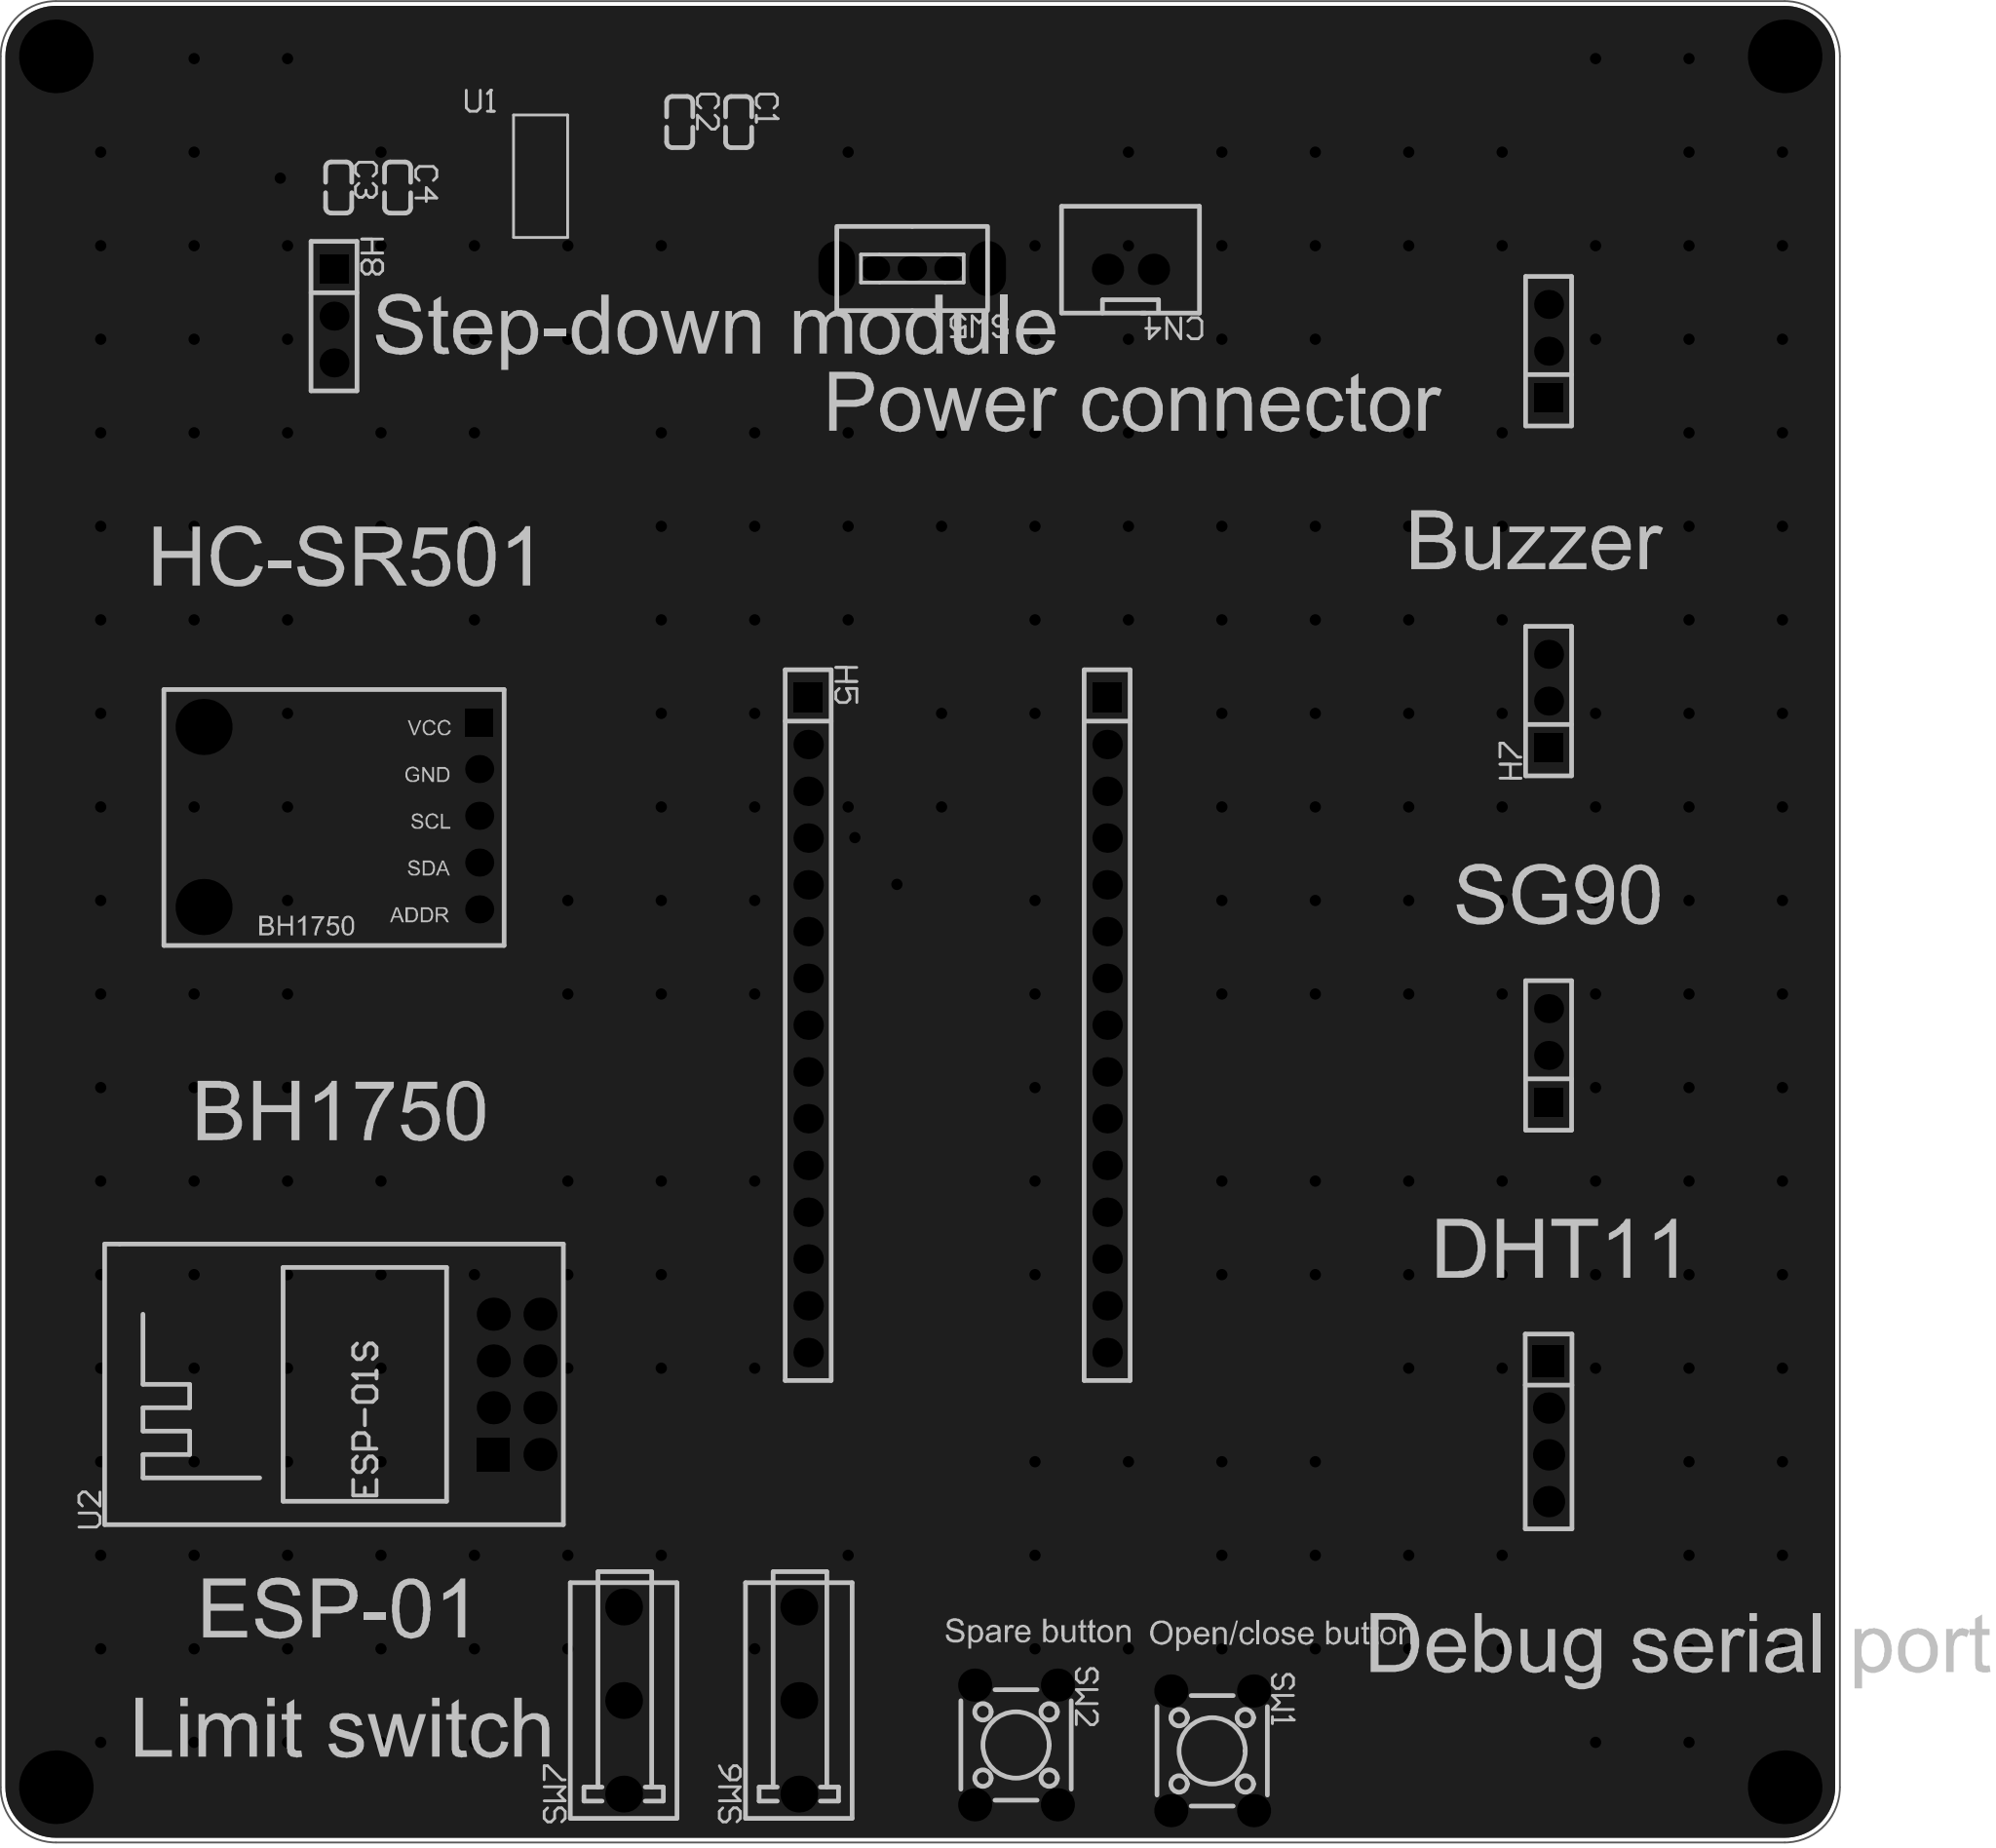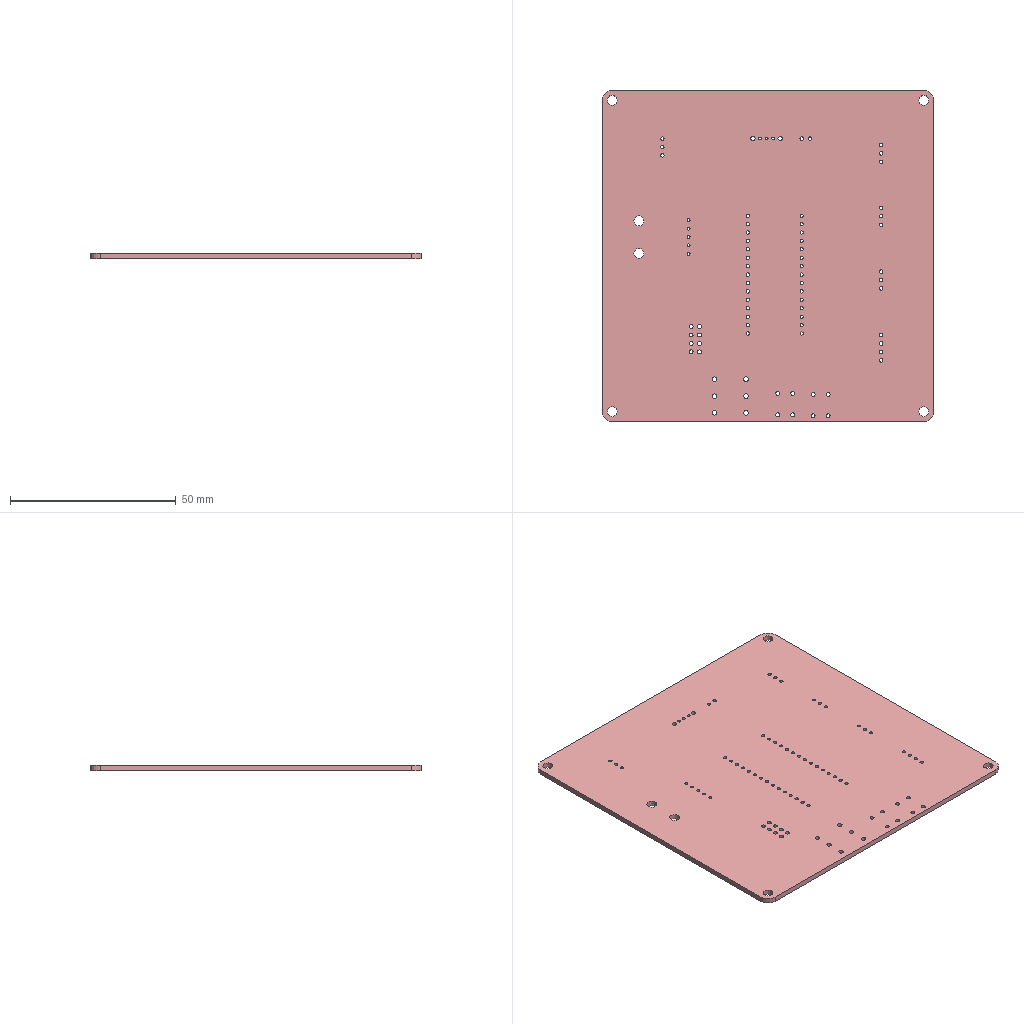Circuit board layout | Altium Designer | box 100 x 100 x 1.6 mm
Layer stack:
# Altium Designer layer stack of  (unit mm; dielectric type: 0 none, 1 core, 2 prepreg, 3 surface material)
index,name,kind,layer,copper_thickness_mm,dielectric_type,dielectric_thickness_mm,dielectric_material,dielectric_constant
0,Top Paste Mask Layer,other,,,,,,
1,Top Silkscreen Layer,other,,,,,,
2,Top Solder Mask Layer,dielectric,,,3,0.01,,3.3
3,Top Layer,copper,Top Layer,0.035,,,,
4,Dielectric1,dielectric,,,3,1.51,FR4,4.5
5,Bottom Layer,copper,Bottom Layer,0.035,,,,
6,Bottom Solder Mask Layer,dielectric,,,3,0.01,,3.3
7,Bottom Silkscreen Layer,other,,,,,,
8,Bottom Paste Mask Layer,other,,,,,,
# drill layer pairs: low layer,high layer
drill_pair,Top Layer,Bottom Layer
Part placement:
Designator,Comment,Layer,Footprint,Center-X(mm),Center-Y(mm),Rotation
SW1,,TopLayer,SW-TH_4P-L6.0-W6.0-P4.50-LS6.5,157.222,85.915,270
SW2,,TopLayer,SW-TH_4P-L6.0-W6.0-P4.50-LS6.5,146.558,86.233,270
H1,,TopLayer,HDR-TH_3P-P2.54-V-F,175.514,161.925,90
H3,,TopLayer,HDR-TH_3P-P2.54-V-F,175.514,123.68,90
U3,,TopLayer,BH1750光照传感器,109.876,136.693,0
H2,,TopLayer,HDR-TH_4P-P2.54-V-F,175.514,103.259,270
H5,,TopLayer,HDR-TH_15P-P2.54-V-F-1,135.255,125.325,270
H7,,TopLayer,HDR-TH_3P-P2.54-V-F,175.514,142.924,90
H8,,TopLayer,HDR-TH_3P-P2.54-V-F,109.474,163.83,270
H6,,TopLayer,HDR-TH_15P-P2.54-V-F-1,151.511,125.325,270
U2,ESP-01S,TopLayer,WIFIM-TH_ESP-01S,119.405,105.817,90
CN4,XH2.54*2P_through-hole,TopLayer,CONN-TH_2P-P2.50-XH2.54-2P,152.781,166.37,180
SW5,,TopLayer,拨动开关,140.912,166.415,180
SW6,DM1-12UP-1,TopLayer,SW-TH_DM1-12UP-1,134.747,88.646,90
SW7,DM1-12UP-1,TopLayer,SW-TH_DM1-12UP-1,125.222,88.646,90
C1,100nF,TopLayer,C0603,131.475,174.369,270
C2,10uF,TopLayer,C0603,128.27,174.371,270
C3,10uF,TopLayer,C0603,109.728,170.815,90
C4,100nF,TopLayer,C0603,112.932,170.814,90
U1,AMS1117-3.3,TopLayer,SOT-223-3_L6.5-W3.4-P2.30-LS7.0-BR,120.806,171.427,0
Pad and via stacks:
# Altium Designer via and pad stacks of  (unit mm). Each distinct definition once, with the count of objects using it.
# via: kind,start_layer,end_layer,hole_mm,diameter_mm,mode(0 simple;1 top-mid-bottom;2 full stack),diameter_per_layer,count,example_net
# pad: kind,layer,hole_mm,hole_type(0 round;1 square;2 slot),plating,top_size,top_shape(1 round;2 rect;3 octagon;9 rounded rect),mid_size,bottom_size,mode,footprint,size_per_layer,count,example
pad,Multi-Layer,3,0,plated,4x4,1,4x4,4x4,0,,,4,1
pad,Multi-Layer,1.2,0,plated,1.8x1.8,1,1.8x1.8,1.8x1.8,0,SW-TH_4P-L6.0-W6.0-P4.50-LS6.5,,8,SW1.1
pad,Multi-Layer,1.02,0,plated,1.575x1.575,1,1.575x1.575,1.575x1.575,0,HDR-TH_3P-P2.54-V-F,,8,H1.3
pad,Multi-Layer,1.02,0,plated,1.575x1.575,2,1.575x1.575,1.575x1.575,0,HDR-TH_3P-P2.54-V-F,,4,H1.1
pad,Multi-Layer,3.048,0,unplated,3.048x3.048,1,3.048x3.048,3.048x3.048,0,BH1750\u00B9\u00E2\u00D5\u00D5\u00B4\u00AB\u00B8\u00D0\u00C6\u00F7,,2,U3.
pad,Multi-Layer,0.9144,0,plated,1.524x1.524,2,1.524x1.524,1.524x1.524,0,BH1750\u00B9\u00E2\u00D5\u00D5\u00B4\u00AB\u00B8\u00D0\u00C6\u00F7,,1,U3.1
pad,Multi-Layer,0.9144,0,plated,1.524x1.524,1,1.524x1.524,1.524x1.524,0,BH1750\u00B9\u00E2\u00D5\u00D5\u00B4\u00AB\u00B8\u00D0\u00C6\u00F7,,4,U3.4
pad,Multi-Layer,1.1,0,plated,1.7x1.7,2,1.7x1.7,1.7x1.7,0,HDR-TH_4P-P2.54-V-F,,1,H2.1
pad,Multi-Layer,1.1,0,plated,1.7x1.7,1,1.7x1.7,1.7x1.7,0,HDR-TH_4P-P2.54-V-F,,3,H2.2
pad,Multi-Layer,1,0,plated,1.6x1.6,1,1.6x1.6,1.6x1.6,0,HDR-TH_15P-P2.54-V-F-1,,28,H5.15
pad,Multi-Layer,1,0,plated,1.6x1.575,2,1.6x1.575,1.6x1.575,0,HDR-TH_15P-P2.54-V-F-1,,2,H5.1
pad,Multi-Layer,1.2,0,plated,1.8x1.8,2,1.8x1.8,1.8x1.8,0,WIFIM-TH_ESP-01S,,1,U2.1
pad,Multi-Layer,1.2,0,plated,1.8x1.8,1,1.8x1.8,1.8x1.8,0,WIFIM-TH_ESP-01S,,7,U2.2
pad,Multi-Layer,1.05,0,plated,1.7x1.7,1,1.7x1.7,1.7x1.7,0,CONN-TH_2P-P2.50-XH2.54-2P,,2,CN4.2
pad,Multi-Layer,0.8992,0,plated,1.6x1.3,1,1.6x1.3,1.6x1.3,0,\u00B2\u00A6\u00B6\u00AF\u00BF\u00AA\u00B9\u00D8,,3,SW5.1
pad,Multi-Layer,1.3,0,plated,3x1.999,1,3x1.999,3x1.999,0,\u00B2\u00A6\u00B6\u00AF\u00BF\u00AA\u00B9\u00D8,,2,SW5.4
pad,Multi-Layer,1.4,0,plated,2x2,1,2x2,2x2,0,SW-TH_DM1-12UP-1,,6,SW6.3
pad,Top Layer,0,0,plated,0.8x0.9,2,0.8x0.9,0.8x0.9,0,C0603,,8,C1.2
pad,Top Layer,0,0,plated,2.5x1.1,2,2.5x1.1,2.5x1.1,0,SOT-223-3_L6.5-W3.4-P2.30-LS7.0-BR,,3,U1.1
pad,Top Layer,0,0,plated,2.34x3.6,2,2.34x3.6,2.34x3.6,0,SOT-223-3_L6.5-W3.4-P2.30-LS7.0-BR,,1,U1.4
via,Top Layer,Bottom Layer,0.3048,0.61,0,,246,D8
Copper pours:
name,layer,net,type(0 solid;1 hatched;2 none)
Bottom Layer-GND,Bottom Layer,GND,0
Top Layer-GND,Top Layer,GND,0
Design rules, without the lines most boards share:
# Altium Designer design rules of  (exported by Altium Designer, unit mm)
# columns: name | kind | enabled | priority | scope1 | scope2 | descriptor | typed fields (field=value)
Copper_copperRegion_copperThickness1oz | 0 | disabled | 4 | All | All | Clearance Constraint (Gap=5.984mil) (Disabled)(All),(All) | gap=0.152
Copper_copperRegion_copperThickness1oz_1 | 63 | disabled | 4 | All | All | Board Clearance Constraint (Gap=0mil) (Disabled)(All) |
Copper_copperRegion_Copper_copperRegion | 0 | disabled | 5 | All | All | Clearance Constraint (Gap=5.984mil) (Disabled)(All),(All) | gap=0.152
Copper_copperRegion_Copper_copperRegion_1 | 63 | disabled | 5 | All | All | Board Clearance Constraint (Gap=0mil) (Disabled)(All) |
copperThickness1oz | 0 | enabled | 6 | All | All | Clearance Constraint (Gap=5.984mil) (All),(All) | gap=0.152
copperThickness1oz_1 | 63 | enabled | 6 | All | All | Board Clearance Constraint (Gap=0mil) (All) |
copperRegion_copperThickness1oz | 20 | disabled | 1 | All | All | Polygon Connect Rule(Relief Connect )(Conductor Width=10mil) (Relief Angle=90 Angle) (Entries=4) (Air Gap Width=10mil) (Disabled)(All),(All) | connect_style(0=relief,1=direct,2=none)=0 relief_conductor_width=0.254 relief_entries=4
copperRegion_Copper_copperRegion | 20 | disabled | 2 | All | All | Polygon Connect Rule(Relief Connect )(Conductor Width=10mil) (Relief Angle=90 Angle) (Entries=4) (Air Gap Width=10mil) (Disabled)(All),(All) | connect_style(0=relief,1=direct,2=none)=0 relief_conductor_width=0.254 relief_entries=4
copperRegion | 20 | enabled | 3 | All | All | Polygon Connect Rule(Relief Connect )(Conductor Width=10mil) (Relief Angle=90 Angle) (Entries=4) (Air Gap Width=10mil) (All),(All) | connect_style(0=relief,1=direct,2=none)=0 relief_conductor_width=0.254 relief_entries=4